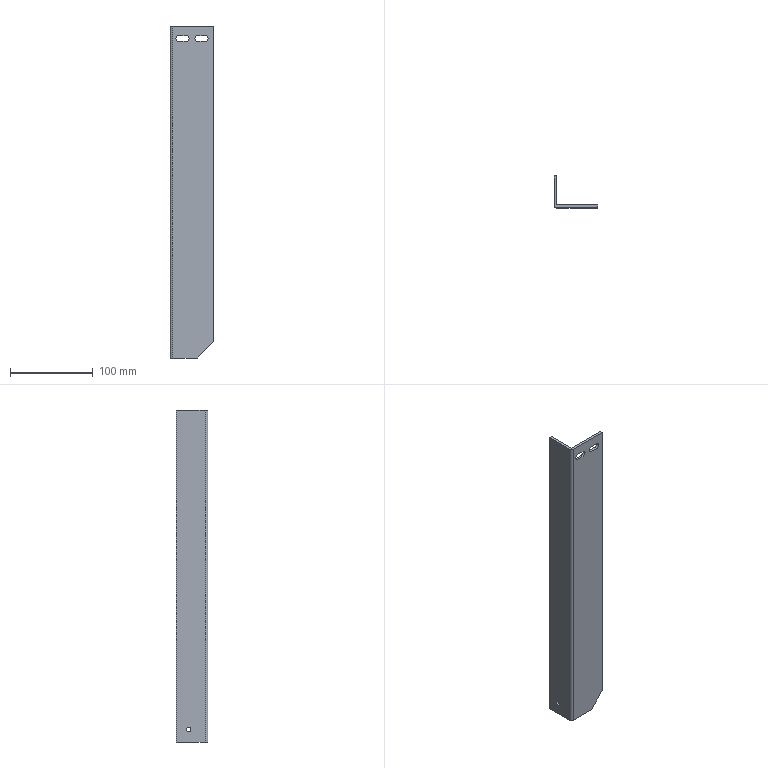Part | STEP file | DT-012 | 1 solid | 21 faces | box 53 x 38 x 400 mm | volume 103503 mm3 | plane 13 | cylinder 8 | commonest cylinder face diameters 7 x4 5.2 x2 0.2 x1 6.2 x1
STEP:
#1=CARTESIAN_POINT('',(-47.404,11.625,12.4));
#2=VERTEX_POINT('',#1);
#3=CARTESIAN_POINT('',(-47.404,11.625,17.6));
#4=VERTEX_POINT('',#3);
#5=CARTESIAN_POINT('',(-47.404,11.625,15.));
#6=DIRECTION('',(-1.,0.,0.));
#7=DIRECTION('',(0.,0.,1.));
#8=AXIS2_PLACEMENT_3D('',#5,#6,#7);
#9=CIRCLE('',#8,2.6);
#10=EDGE_CURVE('',#2,#4,#9,.T.);
#11=ORIENTED_EDGE('',*,*,#10,.F.);
#12=CARTESIAN_POINT('',(-50.404,11.625,12.4));
#13=VERTEX_POINT('',#12);
#14=CARTESIAN_POINT('',(-40.404,11.625,12.4));
#15=DIRECTION('',(-1.,0.,0.));
#16=VECTOR('',#15,1000.);
#17=LINE('',#14,#16);
#18=EDGE_CURVE('',#2,#13,#17,.T.);
#19=ORIENTED_EDGE('',*,*,#18,.T.);
#20=CARTESIAN_POINT('',(-50.404,11.625,17.6));
#21=VERTEX_POINT('',#20);
#22=CARTESIAN_POINT('',(-50.404,11.625,15.));
#23=DIRECTION('',(1.,0.,0.));
#24=DIRECTION('',(0.,0.,1.));
#25=AXIS2_PLACEMENT_3D('',#22,#23,#24);
#26=CIRCLE('',#25,2.6);
#27=EDGE_CURVE('',#21,#13,#26,.T.);
#28=ORIENTED_EDGE('',*,*,#27,.F.);
#29=CARTESIAN_POINT('',(-40.404,11.625,17.6));
#30=DIRECTION('',(-1.,0.,0.));
#31=VECTOR('',#30,1000.);
#32=LINE('',#29,#31);
#33=EDGE_CURVE('',#4,#21,#32,.T.);
#34=ORIENTED_EDGE('',*,*,#33,.F.);
#35=EDGE_LOOP('',(#11,#19,#28,#34));
#36=FACE_OUTER_BOUND('',#35,.T.);
#37=CARTESIAN_POINT('',(-40.404,11.625,15.));
#38=DIRECTION('',(-1.,0.,0.));
#39=DIRECTION('',(0.,0.,1.));
#40=AXIS2_PLACEMENT_3D('',#37,#38,#39);
#41=CYLINDRICAL_SURFACE('',#40,2.6);
#42=ADVANCED_FACE('',(#36),#41,.F.);
#43=CARTESIAN_POINT('',(-47.304,-8.375,0.));
#44=VERTEX_POINT('',#43);
#45=CARTESIAN_POINT('',(-47.304,-8.375,400.));
#46=VERTEX_POINT('',#45);
#47=CARTESIAN_POINT('',(-47.304,-8.375,400.));
#48=DIRECTION('',(0.,0.,1.));
#49=VECTOR('',#48,1000.);
#50=LINE('',#47,#49);
#51=EDGE_CURVE('',#44,#46,#50,.T.);
#52=ORIENTED_EDGE('',*,*,#51,.T.);
#53=CARTESIAN_POINT('',(2.596,-8.375,400.));
#54=VERTEX_POINT('',#53);
#55=CARTESIAN_POINT('',(-47.404,-8.375,400.));
#56=DIRECTION('',(1.,0.,0.));
#57=VECTOR('',#56,1000.);
#58=LINE('',#55,#57);
#59=EDGE_CURVE('',#46,#54,#58,.T.);
#60=ORIENTED_EDGE('',*,*,#59,.T.);
#61=CARTESIAN_POINT('',(2.596,-8.375,20.));
#62=VERTEX_POINT('',#61);
#63=CARTESIAN_POINT('',(2.596,-8.375,400.));
#64=DIRECTION('',(0.,0.,-1.));
#65=VECTOR('',#64,1000.);
#66=LINE('',#63,#65);
#67=EDGE_CURVE('',#54,#62,#66,.T.);
#68=ORIENTED_EDGE('',*,*,#67,.T.);
#69=CARTESIAN_POINT('',(-17.404,-8.375,0.));
#70=VERTEX_POINT('',#69);
#71=CARTESIAN_POINT('',(2.596,-8.375,20.));
#72=DIRECTION('',(-0.7071,0.,-0.7071));
#73=VECTOR('',#72,1000.);
#74=LINE('',#71,#73);
#75=EDGE_CURVE('',#62,#70,#74,.T.);
#76=ORIENTED_EDGE('',*,*,#75,.T.);
#77=CARTESIAN_POINT('',(-47.404,-8.375,0.));
#78=DIRECTION('',(-1.,0.,0.));
#79=VECTOR('',#78,1000.);
#80=LINE('',#77,#79);
#81=EDGE_CURVE('',#70,#44,#80,.T.);
#82=ORIENTED_EDGE('',*,*,#81,.T.);
#83=EDGE_LOOP('',(#52,#60,#68,#76,#82));
#84=FACE_OUTER_BOUND('',#83,.T.);
#85=CARTESIAN_POINT('',(-30.904,-8.375,381.5));
#86=VERTEX_POINT('',#85);
#87=CARTESIAN_POINT('',(-30.904,-8.375,388.5));
#88=VERTEX_POINT('',#87);
#89=CARTESIAN_POINT('',(-30.904,-8.375,385.));
#90=DIRECTION('',(0.,-1.,0.));
#91=DIRECTION('',(0.,0.,1.));
#92=AXIS2_PLACEMENT_3D('',#89,#90,#91);
#93=CIRCLE('',#92,3.5);
#94=EDGE_CURVE('',#86,#88,#93,.T.);
#95=ORIENTED_EDGE('',*,*,#94,.T.);
#96=CARTESIAN_POINT('',(-39.904,-8.375,388.5));
#97=VERTEX_POINT('',#96);
#98=CARTESIAN_POINT('',(-47.404,-8.375,388.5));
#99=DIRECTION('',(-1.,0.,0.));
#100=VECTOR('',#99,1000.);
#101=LINE('',#98,#100);
#102=EDGE_CURVE('',#88,#97,#101,.T.);
#103=ORIENTED_EDGE('',*,*,#102,.T.);
#104=CARTESIAN_POINT('',(-39.904,-8.375,381.5));
#105=VERTEX_POINT('',#104);
#106=CARTESIAN_POINT('',(-39.904,-8.375,385.));
#107=DIRECTION('',(0.,-1.,0.));
#108=DIRECTION('',(0.,0.,1.));
#109=AXIS2_PLACEMENT_3D('',#106,#107,#108);
#110=CIRCLE('',#109,3.5);
#111=EDGE_CURVE('',#97,#105,#110,.T.);
#112=ORIENTED_EDGE('',*,*,#111,.T.);
#113=CARTESIAN_POINT('',(-47.404,-8.375,381.5));
#114=DIRECTION('',(1.,0.,0.));
#115=VECTOR('',#114,1000.);
#116=LINE('',#113,#115);
#117=EDGE_CURVE('',#105,#86,#116,.T.);
#118=ORIENTED_EDGE('',*,*,#117,.T.);
#119=EDGE_LOOP('',(#95,#103,#112,#118));
#120=FACE_BOUND('',#119,.T.);
#121=CARTESIAN_POINT('',(-7.904,-8.375,381.5));
#122=VERTEX_POINT('',#121);
#123=CARTESIAN_POINT('',(-7.904,-8.375,388.5));
#124=VERTEX_POINT('',#123);
#125=CARTESIAN_POINT('',(-7.904,-8.375,385.));
#126=DIRECTION('',(0.,-1.,0.));
#127=DIRECTION('',(0.,0.,1.));
#128=AXIS2_PLACEMENT_3D('',#125,#126,#127);
#129=CIRCLE('',#128,3.5);
#130=EDGE_CURVE('',#122,#124,#129,.T.);
#131=ORIENTED_EDGE('',*,*,#130,.T.);
#132=CARTESIAN_POINT('',(-16.904,-8.375,388.5));
#133=VERTEX_POINT('',#132);
#134=CARTESIAN_POINT('',(-47.404,-8.375,388.5));
#135=DIRECTION('',(-1.,0.,0.));
#136=VECTOR('',#135,1000.);
#137=LINE('',#134,#136);
#138=EDGE_CURVE('',#124,#133,#137,.T.);
#139=ORIENTED_EDGE('',*,*,#138,.T.);
#140=CARTESIAN_POINT('',(-16.904,-8.375,381.5));
#141=VERTEX_POINT('',#140);
#142=CARTESIAN_POINT('',(-16.904,-8.375,385.));
#143=DIRECTION('',(0.,-1.,0.));
#144=DIRECTION('',(0.,0.,1.));
#145=AXIS2_PLACEMENT_3D('',#142,#143,#144);
#146=CIRCLE('',#145,3.5);
#147=EDGE_CURVE('',#133,#141,#146,.T.);
#148=ORIENTED_EDGE('',*,*,#147,.T.);
#149=CARTESIAN_POINT('',(-47.404,-8.375,381.5));
#150=DIRECTION('',(1.,0.,0.));
#151=VECTOR('',#150,1000.);
#152=LINE('',#149,#151);
#153=EDGE_CURVE('',#141,#122,#152,.T.);
#154=ORIENTED_EDGE('',*,*,#153,.T.);
#155=EDGE_LOOP('',(#131,#139,#148,#154));
#156=FACE_BOUND('',#155,.T.);
#157=CARTESIAN_POINT('',(-47.404,-8.375,400.));
#158=DIRECTION('',(0.,1.,0.));
#159=DIRECTION('',(0.,0.,1.));
#160=AXIS2_PLACEMENT_3D('',#157,#158,#159);
#161=PLANE('',#160);
#162=ADVANCED_FACE('',(#84,#120,#156),#161,.T.);
#163=CARTESIAN_POINT('',(-47.304,-11.375,400.));
#164=VERTEX_POINT('',#163);
#165=CARTESIAN_POINT('',(2.596,-11.375,400.));
#166=VERTEX_POINT('',#165);
#167=CARTESIAN_POINT('',(-50.404,-11.375,400.));
#168=DIRECTION('',(1.,0.,0.));
#169=VECTOR('',#168,1000.);
#170=LINE('',#167,#169);
#171=EDGE_CURVE('',#164,#166,#170,.T.);
#172=ORIENTED_EDGE('',*,*,#171,.T.);
#173=CARTESIAN_POINT('',(2.596,-8.275,400.));
#174=DIRECTION('',(0.,1.,0.));
#175=VECTOR('',#174,1000.);
#176=LINE('',#173,#175);
#177=EDGE_CURVE('',#166,#54,#176,.T.);
#178=ORIENTED_EDGE('',*,*,#177,.T.);
#179=ORIENTED_EDGE('',*,*,#59,.F.);
#180=CARTESIAN_POINT('',(-47.404,-8.275,400.));
#181=VERTEX_POINT('',#180);
#182=CARTESIAN_POINT('',(-47.304,-8.275,400.));
#183=DIRECTION('',(0.,0.,-1.));
#184=DIRECTION('',(-1.,0.,0.));
#185=AXIS2_PLACEMENT_3D('',#182,#183,#184);
#186=CIRCLE('',#185,0.1);
#187=EDGE_CURVE('',#46,#181,#186,.T.);
#188=ORIENTED_EDGE('',*,*,#187,.T.);
#189=CARTESIAN_POINT('',(-47.404,26.625,400.));
#190=VERTEX_POINT('',#189);
#191=CARTESIAN_POINT('',(-47.404,26.625,400.));
#192=DIRECTION('',(0.,-1.,0.));
#193=VECTOR('',#192,1000.);
#194=LINE('',#191,#193);
#195=EDGE_CURVE('',#190,#181,#194,.T.);
#196=ORIENTED_EDGE('',*,*,#195,.F.);
#197=CARTESIAN_POINT('',(-50.404,26.625,400.));
#198=VERTEX_POINT('',#197);
#199=CARTESIAN_POINT('',(-47.304,26.625,400.));
#200=DIRECTION('',(1.,0.,0.));
#201=VECTOR('',#200,1000.);
#202=LINE('',#199,#201);
#203=EDGE_CURVE('',#198,#190,#202,.T.);
#204=ORIENTED_EDGE('',*,*,#203,.F.);
#205=CARTESIAN_POINT('',(-50.404,-8.275,400.));
#206=VERTEX_POINT('',#205);
#207=CARTESIAN_POINT('',(-50.404,-8.275,400.));
#208=DIRECTION('',(0.,1.,0.));
#209=VECTOR('',#208,1000.);
#210=LINE('',#207,#209);
#211=EDGE_CURVE('',#206,#198,#210,.T.);
#212=ORIENTED_EDGE('',*,*,#211,.F.);
#213=CARTESIAN_POINT('',(-47.304,-8.275,400.));
#214=DIRECTION('',(0.,0.,1.));
#215=DIRECTION('',(-1.,0.,0.));
#216=AXIS2_PLACEMENT_3D('',#213,#214,#215);
#217=CIRCLE('',#216,3.1);
#218=EDGE_CURVE('',#206,#164,#217,.T.);
#219=ORIENTED_EDGE('',*,*,#218,.T.);
#220=EDGE_LOOP('',(#172,#178,#179,#188,#196,#204,#212,#219));
#221=FACE_OUTER_BOUND('',#220,.T.);
#222=CARTESIAN_POINT('',(-50.404,-8.275,400.));
#223=DIRECTION('',(0.,0.,1.));
#224=DIRECTION('',(1.,0.,0.));
#225=AXIS2_PLACEMENT_3D('',#222,#223,#224);
#226=PLANE('',#225);
#227=ADVANCED_FACE('',(#221),#226,.T.);
#228=CARTESIAN_POINT('',(-47.404,-8.275,0.));
#229=VERTEX_POINT('',#228);
#230=CARTESIAN_POINT('',(-47.404,-8.275,400.));
#231=DIRECTION('',(0.,0.,-1.));
#232=VECTOR('',#231,1000.);
#233=LINE('',#230,#232);
#234=EDGE_CURVE('',#181,#229,#233,.T.);
#235=ORIENTED_EDGE('',*,*,#234,.F.);
#236=ORIENTED_EDGE('',*,*,#187,.F.);
#237=ORIENTED_EDGE('',*,*,#51,.F.);
#238=CARTESIAN_POINT('',(-47.304,-8.275,0.));
#239=DIRECTION('',(0.,0.,1.));
#240=DIRECTION('',(-1.,0.,0.));
#241=AXIS2_PLACEMENT_3D('',#238,#239,#240);
#242=CIRCLE('',#241,0.1);
#243=EDGE_CURVE('',#229,#44,#242,.T.);
#244=ORIENTED_EDGE('',*,*,#243,.F.);
#245=EDGE_LOOP('',(#235,#236,#237,#244));
#246=FACE_OUTER_BOUND('',#245,.T.);
#247=CARTESIAN_POINT('',(-47.304,-8.275,400.));
#248=DIRECTION('',(0.,0.,-1.));
#249=DIRECTION('',(-1.,0.,0.));
#250=AXIS2_PLACEMENT_3D('',#247,#248,#249);
#251=CYLINDRICAL_SURFACE('',#250,0.1);
#252=ADVANCED_FACE('',(#246),#251,.F.);
#253=CARTESIAN_POINT('',(-17.404,-11.375,0.));
#254=VERTEX_POINT('',#253);
#255=CARTESIAN_POINT('',(-47.304,-11.375,0.));
#256=VERTEX_POINT('',#255);
#257=CARTESIAN_POINT('',(-47.304,-11.375,0.));
#258=DIRECTION('',(-1.,0.,0.));
#259=VECTOR('',#258,1000.);
#260=LINE('',#257,#259);
#261=EDGE_CURVE('',#254,#256,#260,.T.);
#262=ORIENTED_EDGE('',*,*,#261,.T.);
#263=CARTESIAN_POINT('',(-50.404,-8.275,0.));
#264=VERTEX_POINT('',#263);
#265=CARTESIAN_POINT('',(-47.304,-8.275,0.));
#266=DIRECTION('',(0.,0.,-1.));
#267=DIRECTION('',(-1.,0.,0.));
#268=AXIS2_PLACEMENT_3D('',#265,#266,#267);
#269=CIRCLE('',#268,3.1);
#270=EDGE_CURVE('',#256,#264,#269,.T.);
#271=ORIENTED_EDGE('',*,*,#270,.T.);
#272=CARTESIAN_POINT('',(-50.404,26.625,0.));
#273=VERTEX_POINT('',#272);
#274=CARTESIAN_POINT('',(-50.404,-11.375,0.));
#275=DIRECTION('',(0.,1.,0.));
#276=VECTOR('',#275,1000.);
#277=LINE('',#274,#276);
#278=EDGE_CURVE('',#264,#273,#277,.T.);
#279=ORIENTED_EDGE('',*,*,#278,.T.);
#280=CARTESIAN_POINT('',(-47.404,26.625,0.));
#281=VERTEX_POINT('',#280);
#282=CARTESIAN_POINT('',(-50.404,26.625,0.));
#283=DIRECTION('',(-1.,0.,0.));
#284=VECTOR('',#283,1000.);
#285=LINE('',#282,#284);
#286=EDGE_CURVE('',#281,#273,#285,.T.);
#287=ORIENTED_EDGE('',*,*,#286,.F.);
#288=CARTESIAN_POINT('',(-47.404,26.625,0.));
#289=DIRECTION('',(0.,1.,0.));
#290=VECTOR('',#289,1000.);
#291=LINE('',#288,#290);
#292=EDGE_CURVE('',#229,#281,#291,.T.);
#293=ORIENTED_EDGE('',*,*,#292,.F.);
#294=ORIENTED_EDGE('',*,*,#243,.T.);
#295=ORIENTED_EDGE('',*,*,#81,.F.);
#296=CARTESIAN_POINT('',(-17.404,-8.275,0.));
#297=DIRECTION('',(0.,-1.,0.));
#298=VECTOR('',#297,1000.);
#299=LINE('',#296,#298);
#300=EDGE_CURVE('',#70,#254,#299,.T.);
#301=ORIENTED_EDGE('',*,*,#300,.T.);
#302=EDGE_LOOP('',(#262,#271,#279,#287,#293,#294,#295,#301));
#303=FACE_OUTER_BOUND('',#302,.T.);
#304=CARTESIAN_POINT('',(-47.304,-8.275,0.));
#305=DIRECTION('',(0.,0.,-1.));
#306=DIRECTION('',(-1.,0.,0.));
#307=AXIS2_PLACEMENT_3D('',#304,#305,#306);
#308=PLANE('',#307);
#309=ADVANCED_FACE('',(#303),#308,.T.);
#310=CARTESIAN_POINT('',(2.596,-11.375,20.));
#311=VERTEX_POINT('',#310);
#312=CARTESIAN_POINT('',(2.596,-8.275,20.));
#313=DIRECTION('',(0.,1.,0.));
#314=VECTOR('',#313,1000.);
#315=LINE('',#312,#314);
#316=EDGE_CURVE('',#311,#62,#315,.T.);
#317=ORIENTED_EDGE('',*,*,#316,.F.);
#318=CARTESIAN_POINT('',(-17.404,-11.375,0.));
#319=DIRECTION('',(0.7071,0.,0.7071));
#320=VECTOR('',#319,1000.);
#321=LINE('',#318,#320);
#322=EDGE_CURVE('',#254,#311,#321,.T.);
#323=ORIENTED_EDGE('',*,*,#322,.F.);
#324=ORIENTED_EDGE('',*,*,#300,.F.);
#325=ORIENTED_EDGE('',*,*,#75,.F.);
#326=EDGE_LOOP('',(#317,#323,#324,#325));
#327=FACE_OUTER_BOUND('',#326,.T.);
#328=CARTESIAN_POINT('',(-17.404,-8.275,0.));
#329=DIRECTION('',(-0.7071,0.,0.7071));
#330=DIRECTION('',(0.7071,0.,0.7071));
#331=AXIS2_PLACEMENT_3D('',#328,#329,#330);
#332=PLANE('',#331);
#333=ADVANCED_FACE('',(#327),#332,.F.);
#334=ORIENTED_EDGE('',*,*,#67,.F.);
#335=ORIENTED_EDGE('',*,*,#177,.F.);
#336=CARTESIAN_POINT('',(2.596,-11.375,400.));
#337=DIRECTION('',(0.,0.,-1.));
#338=VECTOR('',#337,1000.);
#339=LINE('',#336,#338);
#340=EDGE_CURVE('',#166,#311,#339,.T.);
#341=ORIENTED_EDGE('',*,*,#340,.T.);
#342=ORIENTED_EDGE('',*,*,#316,.T.);
#343=EDGE_LOOP('',(#334,#335,#341,#342));
#344=FACE_OUTER_BOUND('',#343,.T.);
#345=CARTESIAN_POINT('',(2.596,-8.375,400.));
#346=DIRECTION('',(1.,0.,0.));
#347=DIRECTION('',(0.,0.,-1.));
#348=AXIS2_PLACEMENT_3D('',#345,#346,#347);
#349=PLANE('',#348);
#350=ADVANCED_FACE('',(#344),#349,.T.);
#351=ORIENTED_EDGE('',*,*,#102,.F.);
#352=CARTESIAN_POINT('',(-30.904,-11.375,388.5));
#353=VERTEX_POINT('',#352);
#354=CARTESIAN_POINT('',(-30.904,-18.375,388.5));
#355=DIRECTION('',(0.,1.,0.));
#356=VECTOR('',#355,1000.);
#357=LINE('',#354,#356);
#358=EDGE_CURVE('',#353,#88,#357,.T.);
#359=ORIENTED_EDGE('',*,*,#358,.F.);
#360=CARTESIAN_POINT('',(-39.904,-11.375,388.5));
#361=VERTEX_POINT('',#360);
#362=CARTESIAN_POINT('',(-39.904,-11.375,388.5));
#363=DIRECTION('',(1.,0.,0.));
#364=VECTOR('',#363,1000.);
#365=LINE('',#362,#364);
#366=EDGE_CURVE('',#361,#353,#365,.T.);
#367=ORIENTED_EDGE('',*,*,#366,.F.);
#368=CARTESIAN_POINT('',(-39.904,-18.375,388.5));
#369=DIRECTION('',(0.,-1.,0.));
#370=VECTOR('',#369,1000.);
#371=LINE('',#368,#370);
#372=EDGE_CURVE('',#97,#361,#371,.T.);
#373=ORIENTED_EDGE('',*,*,#372,.F.);
#374=EDGE_LOOP('',(#351,#359,#367,#373));
#375=FACE_OUTER_BOUND('',#374,.T.);
#376=CARTESIAN_POINT('',(-39.904,-18.375,388.5));
#377=DIRECTION('',(0.,0.,1.));
#378=DIRECTION('',(1.,0.,0.));
#379=AXIS2_PLACEMENT_3D('',#376,#377,#378);
#380=PLANE('',#379);
#381=ADVANCED_FACE('',(#375),#380,.F.);
#382=ORIENTED_EDGE('',*,*,#94,.F.);
#383=CARTESIAN_POINT('',(-30.904,-11.375,381.5));
#384=VERTEX_POINT('',#383);
#385=CARTESIAN_POINT('',(-30.904,-18.375,381.5));
#386=DIRECTION('',(0.,1.,0.));
#387=VECTOR('',#386,1000.);
#388=LINE('',#385,#387);
#389=EDGE_CURVE('',#384,#86,#388,.T.);
#390=ORIENTED_EDGE('',*,*,#389,.F.);
#391=CARTESIAN_POINT('',(-30.904,-11.375,385.));
#392=DIRECTION('',(0.,1.,0.));
#393=DIRECTION('',(0.,0.,1.));
#394=AXIS2_PLACEMENT_3D('',#391,#392,#393);
#395=CIRCLE('',#394,3.5);
#396=EDGE_CURVE('',#353,#384,#395,.T.);
#397=ORIENTED_EDGE('',*,*,#396,.F.);
#398=ORIENTED_EDGE('',*,*,#358,.T.);
#399=EDGE_LOOP('',(#382,#390,#397,#398));
#400=FACE_OUTER_BOUND('',#399,.T.);
#401=CARTESIAN_POINT('',(-30.904,-18.375,385.));
#402=DIRECTION('',(0.,1.,0.));
#403=DIRECTION('',(0.,0.,1.));
#404=AXIS2_PLACEMENT_3D('',#401,#402,#403);
#405=CYLINDRICAL_SURFACE('',#404,3.5);
#406=ADVANCED_FACE('',(#400),#405,.F.);
#407=ORIENTED_EDGE('',*,*,#117,.F.);
#408=CARTESIAN_POINT('',(-39.904,-11.375,381.5));
#409=VERTEX_POINT('',#408);
#410=CARTESIAN_POINT('',(-39.904,-18.375,381.5));
#411=DIRECTION('',(0.,1.,0.));
#412=VECTOR('',#411,1000.);
#413=LINE('',#410,#412);
#414=EDGE_CURVE('',#409,#105,#413,.T.);
#415=ORIENTED_EDGE('',*,*,#414,.F.);
#416=CARTESIAN_POINT('',(-39.904,-11.375,381.5));
#417=DIRECTION('',(-1.,0.,0.));
#418=VECTOR('',#417,1000.);
#419=LINE('',#416,#418);
#420=EDGE_CURVE('',#384,#409,#419,.T.);
#421=ORIENTED_EDGE('',*,*,#420,.F.);
#422=ORIENTED_EDGE('',*,*,#389,.T.);
#423=EDGE_LOOP('',(#407,#415,#421,#422));
#424=FACE_OUTER_BOUND('',#423,.T.);
#425=CARTESIAN_POINT('',(-39.904,-18.375,381.5));
#426=DIRECTION('',(0.,0.,-1.));
#427=DIRECTION('',(-1.,0.,0.));
#428=AXIS2_PLACEMENT_3D('',#425,#426,#427);
#429=PLANE('',#428);
#430=ADVANCED_FACE('',(#424),#429,.F.);
#431=ORIENTED_EDGE('',*,*,#111,.F.);
#432=ORIENTED_EDGE('',*,*,#372,.T.);
#433=CARTESIAN_POINT('',(-39.904,-11.375,385.));
#434=DIRECTION('',(0.,1.,0.));
#435=DIRECTION('',(0.,0.,1.));
#436=AXIS2_PLACEMENT_3D('',#433,#434,#435);
#437=CIRCLE('',#436,3.5);
#438=EDGE_CURVE('',#409,#361,#437,.T.);
#439=ORIENTED_EDGE('',*,*,#438,.F.);
#440=ORIENTED_EDGE('',*,*,#414,.T.);
#441=EDGE_LOOP('',(#431,#432,#439,#440));
#442=FACE_OUTER_BOUND('',#441,.T.);
#443=CARTESIAN_POINT('',(-39.904,-18.375,385.));
#444=DIRECTION('',(0.,1.,0.));
#445=DIRECTION('',(0.,0.,1.));
#446=AXIS2_PLACEMENT_3D('',#443,#444,#445);
#447=CYLINDRICAL_SURFACE('',#446,3.5);
#448=ADVANCED_FACE('',(#442),#447,.F.);
#449=ORIENTED_EDGE('',*,*,#138,.F.);
#450=CARTESIAN_POINT('',(-7.904,-11.375,388.5));
#451=VERTEX_POINT('',#450);
#452=CARTESIAN_POINT('',(-7.904,-18.375,388.5));
#453=DIRECTION('',(0.,1.,0.));
#454=VECTOR('',#453,1000.);
#455=LINE('',#452,#454);
#456=EDGE_CURVE('',#451,#124,#455,.T.);
#457=ORIENTED_EDGE('',*,*,#456,.F.);
#458=CARTESIAN_POINT('',(-16.904,-11.375,388.5));
#459=VERTEX_POINT('',#458);
#460=CARTESIAN_POINT('',(-16.904,-11.375,388.5));
#461=DIRECTION('',(1.,0.,0.));
#462=VECTOR('',#461,1000.);
#463=LINE('',#460,#462);
#464=EDGE_CURVE('',#459,#451,#463,.T.);
#465=ORIENTED_EDGE('',*,*,#464,.F.);
#466=CARTESIAN_POINT('',(-16.904,-18.375,388.5));
#467=DIRECTION('',(0.,-1.,0.));
#468=VECTOR('',#467,1000.);
#469=LINE('',#466,#468);
#470=EDGE_CURVE('',#133,#459,#469,.T.);
#471=ORIENTED_EDGE('',*,*,#470,.F.);
#472=EDGE_LOOP('',(#449,#457,#465,#471));
#473=FACE_OUTER_BOUND('',#472,.T.);
#474=CARTESIAN_POINT('',(-16.904,-18.375,388.5));
#475=DIRECTION('',(0.,0.,1.));
#476=DIRECTION('',(1.,0.,0.));
#477=AXIS2_PLACEMENT_3D('',#474,#475,#476);
#478=PLANE('',#477);
#479=ADVANCED_FACE('',(#473),#478,.F.);
#480=ORIENTED_EDGE('',*,*,#130,.F.);
#481=CARTESIAN_POINT('',(-7.904,-11.375,381.5));
#482=VERTEX_POINT('',#481);
#483=CARTESIAN_POINT('',(-7.904,-18.375,381.5));
#484=DIRECTION('',(0.,1.,0.));
#485=VECTOR('',#484,1000.);
#486=LINE('',#483,#485);
#487=EDGE_CURVE('',#482,#122,#486,.T.);
#488=ORIENTED_EDGE('',*,*,#487,.F.);
#489=CARTESIAN_POINT('',(-7.904,-11.375,385.));
#490=DIRECTION('',(0.,1.,0.));
#491=DIRECTION('',(0.,0.,1.));
#492=AXIS2_PLACEMENT_3D('',#489,#490,#491);
#493=CIRCLE('',#492,3.5);
#494=EDGE_CURVE('',#451,#482,#493,.T.);
#495=ORIENTED_EDGE('',*,*,#494,.F.);
#496=ORIENTED_EDGE('',*,*,#456,.T.);
#497=EDGE_LOOP('',(#480,#488,#495,#496));
#498=FACE_OUTER_BOUND('',#497,.T.);
#499=CARTESIAN_POINT('',(-7.904,-18.375,385.));
#500=DIRECTION('',(0.,1.,0.));
#501=DIRECTION('',(0.,0.,1.));
#502=AXIS2_PLACEMENT_3D('',#499,#500,#501);
#503=CYLINDRICAL_SURFACE('',#502,3.5);
#504=ADVANCED_FACE('',(#498),#503,.F.);
#505=ORIENTED_EDGE('',*,*,#153,.F.);
#506=CARTESIAN_POINT('',(-16.904,-11.375,381.5));
#507=VERTEX_POINT('',#506);
#508=CARTESIAN_POINT('',(-16.904,-18.375,381.5));
#509=DIRECTION('',(0.,1.,0.));
#510=VECTOR('',#509,1000.);
#511=LINE('',#508,#510);
#512=EDGE_CURVE('',#507,#141,#511,.T.);
#513=ORIENTED_EDGE('',*,*,#512,.F.);
#514=CARTESIAN_POINT('',(-16.904,-11.375,381.5));
#515=DIRECTION('',(-1.,0.,0.));
#516=VECTOR('',#515,1000.);
#517=LINE('',#514,#516);
#518=EDGE_CURVE('',#482,#507,#517,.T.);
#519=ORIENTED_EDGE('',*,*,#518,.F.);
#520=ORIENTED_EDGE('',*,*,#487,.T.);
#521=EDGE_LOOP('',(#505,#513,#519,#520));
#522=FACE_OUTER_BOUND('',#521,.T.);
#523=CARTESIAN_POINT('',(-16.904,-18.375,381.5));
#524=DIRECTION('',(0.,0.,-1.));
#525=DIRECTION('',(-1.,0.,0.));
#526=AXIS2_PLACEMENT_3D('',#523,#524,#525);
#527=PLANE('',#526);
#528=ADVANCED_FACE('',(#522),#527,.F.);
#529=ORIENTED_EDGE('',*,*,#147,.F.);
#530=ORIENTED_EDGE('',*,*,#470,.T.);
#531=CARTESIAN_POINT('',(-16.904,-11.375,385.));
#532=DIRECTION('',(0.,1.,0.));
#533=DIRECTION('',(0.,0.,1.));
#534=AXIS2_PLACEMENT_3D('',#531,#532,#533);
#535=CIRCLE('',#534,3.5);
#536=EDGE_CURVE('',#507,#459,#535,.T.);
#537=ORIENTED_EDGE('',*,*,#536,.F.);
#538=ORIENTED_EDGE('',*,*,#512,.T.);
#539=EDGE_LOOP('',(#529,#530,#537,#538));
#540=FACE_OUTER_BOUND('',#539,.T.);
#541=CARTESIAN_POINT('',(-16.904,-18.375,385.));
#542=DIRECTION('',(0.,1.,0.));
#543=DIRECTION('',(0.,0.,1.));
#544=AXIS2_PLACEMENT_3D('',#541,#542,#543);
#545=CYLINDRICAL_SURFACE('',#544,3.5);
#546=ADVANCED_FACE('',(#540),#545,.F.);
#547=ORIENTED_EDGE('',*,*,#322,.T.);
#548=ORIENTED_EDGE('',*,*,#340,.F.);
#549=ORIENTED_EDGE('',*,*,#171,.F.);
#550=CARTESIAN_POINT('',(-47.304,-11.375,400.));
#551=DIRECTION('',(0.,0.,1.));
#552=VECTOR('',#551,1000.);
#553=LINE('',#550,#552);
#554=EDGE_CURVE('',#256,#164,#553,.T.);
#555=ORIENTED_EDGE('',*,*,#554,.F.);
#556=ORIENTED_EDGE('',*,*,#261,.F.);
#557=EDGE_LOOP('',(#547,#548,#549,#555,#556));
#558=FACE_OUTER_BOUND('',#557,.T.);
#559=ORIENTED_EDGE('',*,*,#438,.T.);
#560=ORIENTED_EDGE('',*,*,#366,.T.);
#561=ORIENTED_EDGE('',*,*,#396,.T.);
#562=ORIENTED_EDGE('',*,*,#420,.T.);
#563=EDGE_LOOP('',(#559,#560,#561,#562));
#564=FACE_BOUND('',#563,.T.);
#565=ORIENTED_EDGE('',*,*,#536,.T.);
#566=ORIENTED_EDGE('',*,*,#464,.T.);
#567=ORIENTED_EDGE('',*,*,#494,.T.);
#568=ORIENTED_EDGE('',*,*,#518,.T.);
#569=EDGE_LOOP('',(#565,#566,#567,#568));
#570=FACE_BOUND('',#569,.T.);
#571=CARTESIAN_POINT('',(-47.404,-11.375,400.));
#572=DIRECTION('',(0.,1.,0.));
#573=DIRECTION('',(0.,0.,1.));
#574=AXIS2_PLACEMENT_3D('',#571,#572,#573);
#575=PLANE('',#574);
#576=ADVANCED_FACE('',(#558,#564,#570),#575,.F.);
#577=ORIENTED_EDGE('',*,*,#195,.T.);
#578=ORIENTED_EDGE('',*,*,#234,.T.);
#579=ORIENTED_EDGE('',*,*,#292,.T.);
#580=CARTESIAN_POINT('',(-47.404,26.625,400.));
#581=DIRECTION('',(0.,0.,1.));
#582=VECTOR('',#581,1000.);
#583=LINE('',#580,#582);
#584=EDGE_CURVE('',#281,#190,#583,.T.);
#585=ORIENTED_EDGE('',*,*,#584,.T.);
#586=EDGE_LOOP('',(#577,#578,#579,#585));
#587=FACE_OUTER_BOUND('',#586,.T.);
#588=CARTESIAN_POINT('',(-47.404,11.625,15.));
#589=DIRECTION('',(-1.,0.,0.));
#590=DIRECTION('',(0.,0.,1.));
#591=AXIS2_PLACEMENT_3D('',#588,#589,#590);
#592=CIRCLE('',#591,2.6);
#593=EDGE_CURVE('',#4,#2,#592,.T.);
#594=ORIENTED_EDGE('',*,*,#593,.T.);
#595=ORIENTED_EDGE('',*,*,#10,.T.);
#596=EDGE_LOOP('',(#594,#595));
#597=FACE_BOUND('',#596,.T.);
#598=CARTESIAN_POINT('',(-47.404,26.625,400.));
#599=DIRECTION('',(1.,0.,0.));
#600=DIRECTION('',(0.,0.,-1.));
#601=AXIS2_PLACEMENT_3D('',#598,#599,#600);
#602=PLANE('',#601);
#603=ADVANCED_FACE('',(#587,#597),#602,.T.);
#604=ORIENTED_EDGE('',*,*,#218,.F.);
#605=CARTESIAN_POINT('',(-50.404,-8.275,400.));
#606=DIRECTION('',(0.,0.,-1.));
#607=VECTOR('',#606,1000.);
#608=LINE('',#605,#607);
#609=EDGE_CURVE('',#206,#264,#608,.T.);
#610=ORIENTED_EDGE('',*,*,#609,.T.);
#611=ORIENTED_EDGE('',*,*,#270,.F.);
#612=ORIENTED_EDGE('',*,*,#554,.T.);
#613=EDGE_LOOP('',(#604,#610,#611,#612));
#614=FACE_OUTER_BOUND('',#613,.T.);
#615=CARTESIAN_POINT('',(-47.304,-8.275,400.));
#616=DIRECTION('',(0.,0.,-1.));
#617=DIRECTION('',(-1.,0.,0.));
#618=AXIS2_PLACEMENT_3D('',#615,#616,#617);
#619=CYLINDRICAL_SURFACE('',#618,3.1);
#620=ADVANCED_FACE('',(#614),#619,.T.);
#621=ORIENTED_EDGE('',*,*,#203,.T.);
#622=ORIENTED_EDGE('',*,*,#584,.F.);
#623=ORIENTED_EDGE('',*,*,#286,.T.);
#624=CARTESIAN_POINT('',(-50.404,26.625,400.));
#625=DIRECTION('',(0.,0.,1.));
#626=VECTOR('',#625,1000.);
#627=LINE('',#624,#626);
#628=EDGE_CURVE('',#273,#198,#627,.T.);
#629=ORIENTED_EDGE('',*,*,#628,.T.);
#630=EDGE_LOOP('',(#621,#622,#623,#629));
#631=FACE_OUTER_BOUND('',#630,.T.);
#632=CARTESIAN_POINT('',(-50.404,26.625,400.));
#633=DIRECTION('',(0.,1.,0.));
#634=DIRECTION('',(0.,0.,1.));
#635=AXIS2_PLACEMENT_3D('',#632,#633,#634);
#636=PLANE('',#635);
#637=ADVANCED_FACE('',(#631),#636,.T.);
#638=ORIENTED_EDGE('',*,*,#18,.F.);
#639=ORIENTED_EDGE('',*,*,#593,.F.);
#640=ORIENTED_EDGE('',*,*,#33,.T.);
#641=CARTESIAN_POINT('',(-50.404,11.625,15.));
#642=DIRECTION('',(1.,0.,0.));
#643=DIRECTION('',(0.,0.,1.));
#644=AXIS2_PLACEMENT_3D('',#641,#642,#643);
#645=CIRCLE('',#644,2.6);
#646=EDGE_CURVE('',#13,#21,#645,.T.);
#647=ORIENTED_EDGE('',*,*,#646,.F.);
#648=EDGE_LOOP('',(#638,#639,#640,#647));
#649=FACE_OUTER_BOUND('',#648,.T.);
#650=CARTESIAN_POINT('',(-40.404,11.625,15.));
#651=DIRECTION('',(-1.,0.,0.));
#652=DIRECTION('',(0.,0.,1.));
#653=AXIS2_PLACEMENT_3D('',#650,#651,#652);
#654=CYLINDRICAL_SURFACE('',#653,2.6);
#655=ADVANCED_FACE('',(#649),#654,.F.);
#656=ORIENTED_EDGE('',*,*,#609,.F.);
#657=ORIENTED_EDGE('',*,*,#211,.T.);
#658=ORIENTED_EDGE('',*,*,#628,.F.);
#659=ORIENTED_EDGE('',*,*,#278,.F.);
#660=EDGE_LOOP('',(#656,#657,#658,#659));
#661=FACE_OUTER_BOUND('',#660,.T.);
#662=ORIENTED_EDGE('',*,*,#27,.T.);
#663=ORIENTED_EDGE('',*,*,#646,.T.);
#664=EDGE_LOOP('',(#662,#663));
#665=FACE_BOUND('',#664,.T.);
#666=CARTESIAN_POINT('',(-50.404,26.625,400.));
#667=DIRECTION('',(1.,0.,0.));
#668=DIRECTION('',(0.,0.,-1.));
#669=AXIS2_PLACEMENT_3D('',#666,#667,#668);
#670=PLANE('',#669);
#671=ADVANCED_FACE('',(#661,#665),#670,.F.);
#672=CLOSED_SHELL('',(#42,#162,#227,#252,#309,#333,#350,#381,#406,#430,#448,#479,#504,#528,#546,#576,#603,#620,#637,#655,#671));
#673=MANIFOLD_SOLID_BREP('',#672);
#674=CARTESIAN_POINT('',(0.,0.,0.));
#675=DIRECTION('',(0.,0.,1.));
#676=DIRECTION('',(1.,0.,0.));
#677=AXIS2_PLACEMENT_3D('',#674,#675,#676);
#678=(LENGTH_UNIT()NAMED_UNIT(*)SI_UNIT(.MILLI.,.METRE.));
#679=UNCERTAINTY_MEASURE_WITH_UNIT(LENGTH_MEASURE(0.00001),#678,'','');
#680=(NAMED_UNIT(*)PLANE_ANGLE_UNIT()SI_UNIT($,.RADIAN.));
#681=(NAMED_UNIT(*)SI_UNIT($,.STERADIAN.)SOLID_ANGLE_UNIT());
#682=(GEOMETRIC_REPRESENTATION_CONTEXT(3)GLOBAL_UNCERTAINTY_ASSIGNED_CONTEXT((#679))GLOBAL_UNIT_ASSIGNED_CONTEXT((#678,#680,#681))REPRESENTATION_CONTEXT('',''));
#683=ADVANCED_BREP_SHAPE_REPRESENTATION('',(#673,#677),#682);